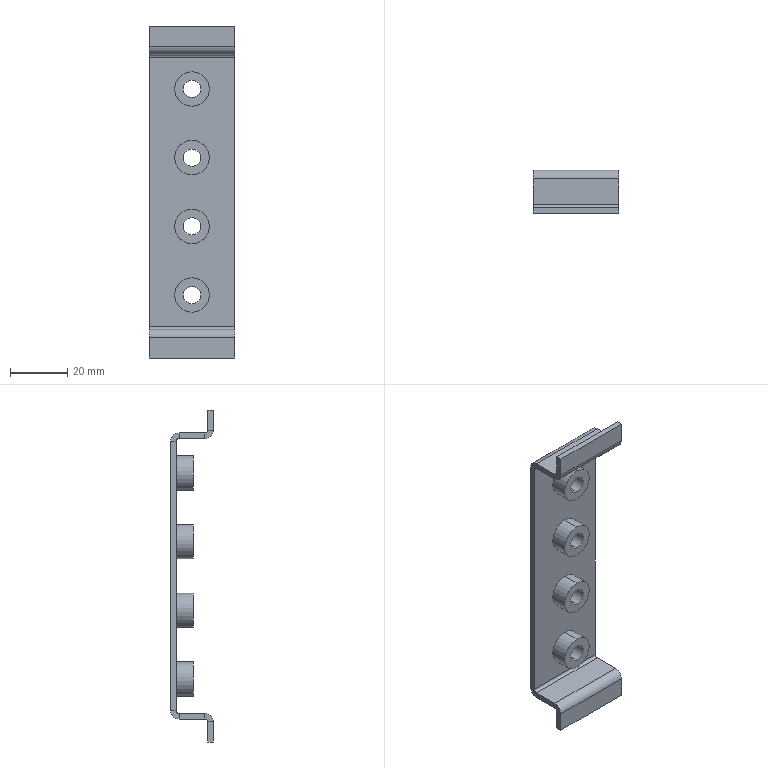Part | SolidWorks | features BaseBody 1 | 1 solid | 70 faces | box 30 x 15 x 116 mm | volume 10084 mm3 | plane 38 | cylinder 32 | commonest cylinder face diameters 6 x12 6.5 x8 12 x8 2 x4